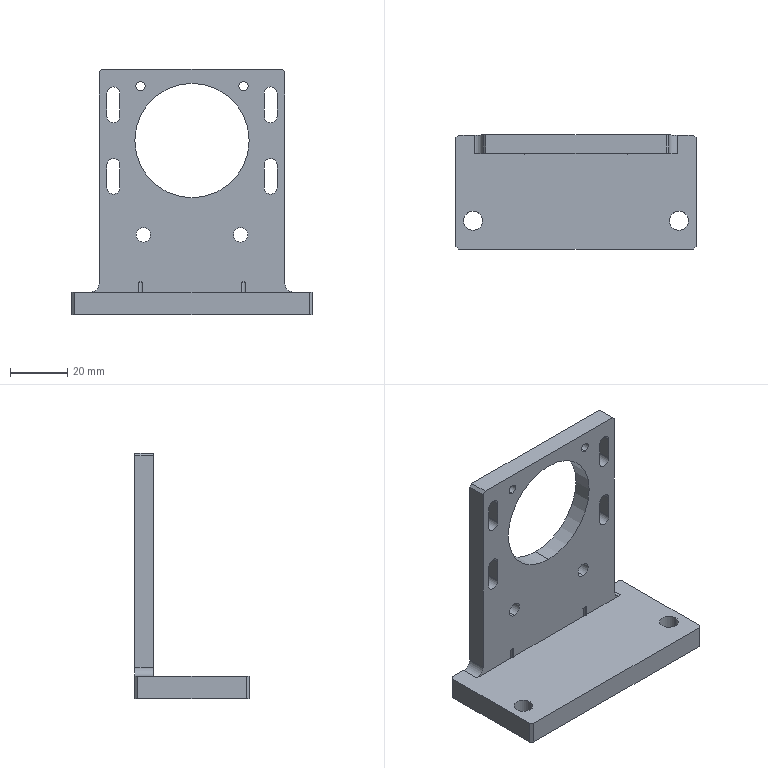Part | STEP file | Motor adapter plate A | 1 solid | 60 faces | box 84 x 40 x 86 mm | volume 49205 mm3 | cylinder 32 | plane 24 | cone 4 | commonest cylinder face diameters 4.5 x12 3.3 x8 5 x4 6.6 x4 6 x2 40 x2